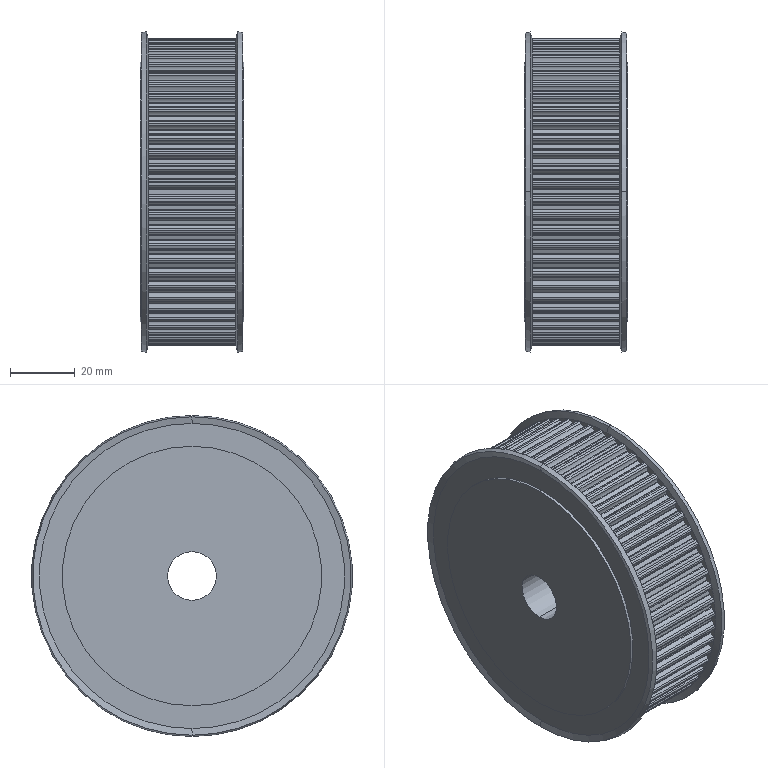Part | SolidWorks | 1 solid | 622 faces | box 32 x 99 x 99 mm | volume 209787 mm3 | cylinder 486 | plane 124 | cone 12 | commonest cylinder face diameters 0.5 x120 1.1 x120 6.55 x120 90.99 x60 94.53 x60 80 x4